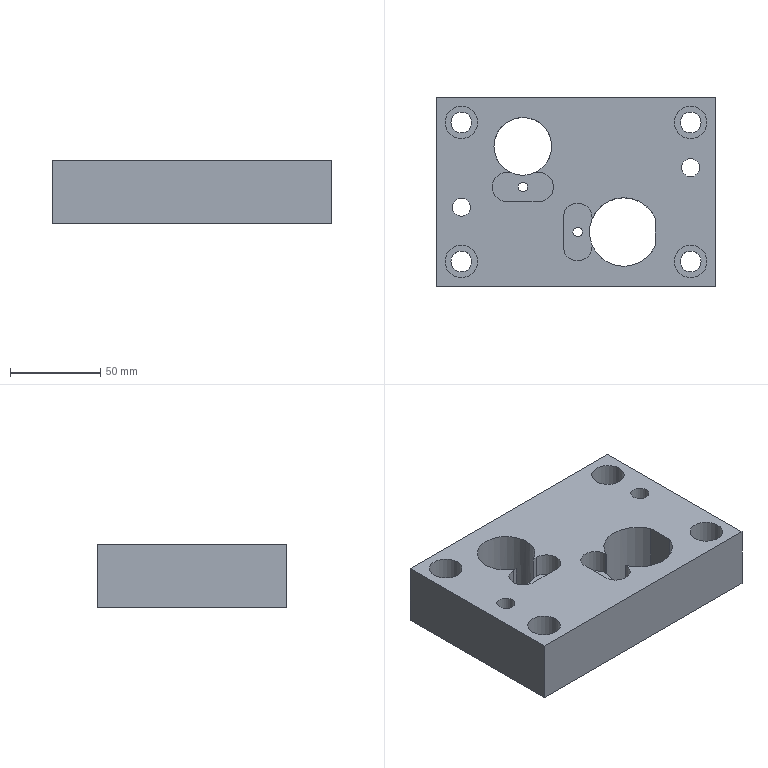Part | STEP file | lll_id4666_x_t | 1 solid | 38 faces | box 155 x 105 x 35 mm | volume 461543 mm3 | plane 19 | cylinder 19 | commonest cylinder face diameters 11.509 x4 16 x4 18.008 x4 5.206 x2 10 x2 38 x2
STEP:
#1=CARTESIAN_POINT('',(475.37,-354.819,-13.));
#2=VERTEX_POINT('',#1);
#3=CARTESIAN_POINT('',(474.87,-353.503,-13.));
#4=VERTEX_POINT('',#3);
#5=CARTESIAN_POINT('',(492.87,-347.42,-13.));
#6=DIRECTION('',(0.,0.,-1.));
#7=DIRECTION('',(1.,0.,0.));
#8=AXIS2_PLACEMENT_3D('',#5,#6,#7);
#9=CIRCLE('',#8,19.);
#10=EDGE_CURVE('',#2,#4,#9,.T.);
#11=ORIENTED_EDGE('',*,*,#10,.T.);
#12=CARTESIAN_POINT('',(475.37,-340.021,-13.));
#13=VERTEX_POINT('',#12);
#14=CARTESIAN_POINT('',(492.87,-347.42,-13.));
#15=DIRECTION('',(0.,0.,-1.));
#16=DIRECTION('',(1.,0.,0.));
#17=AXIS2_PLACEMENT_3D('',#14,#15,#16);
#18=CIRCLE('',#17,19.);
#19=EDGE_CURVE('',#4,#13,#18,.T.);
#20=ORIENTED_EDGE('',*,*,#19,.T.);
#21=CARTESIAN_POINT('',(475.37,-339.42,-13.));
#22=VERTEX_POINT('',#21);
#23=CARTESIAN_POINT('',(475.37,-339.42,-13.));
#24=DIRECTION('',(0.,1.,0.));
#25=VECTOR('',#24,1.);
#26=LINE('',#23,#25);
#27=EDGE_CURVE('',#13,#22,#26,.T.);
#28=ORIENTED_EDGE('',*,*,#27,.T.);
#29=CARTESIAN_POINT('',(459.37,-339.42,-13.));
#30=VERTEX_POINT('',#29);
#31=CARTESIAN_POINT('',(467.37,-339.42,-13.));
#32=DIRECTION('',(0.,0.,-1.));
#33=DIRECTION('',(1.,0.,0.));
#34=AXIS2_PLACEMENT_3D('',#31,#32,#33);
#35=CIRCLE('',#34,8.);
#36=EDGE_CURVE('',#30,#22,#35,.T.);
#37=ORIENTED_EDGE('',*,*,#36,.F.);
#38=CARTESIAN_POINT('',(459.37,-355.42,-13.));
#39=VERTEX_POINT('',#38);
#40=CARTESIAN_POINT('',(459.37,-339.42,-13.));
#41=DIRECTION('',(0.,1.,0.));
#42=VECTOR('',#41,1.);
#43=LINE('',#40,#42);
#44=EDGE_CURVE('',#39,#30,#43,.T.);
#45=ORIENTED_EDGE('',*,*,#44,.F.);
#46=CARTESIAN_POINT('',(475.37,-355.42,-13.));
#47=VERTEX_POINT('',#46);
#48=CARTESIAN_POINT('',(467.37,-355.42,-13.));
#49=DIRECTION('',(0.,0.,-1.));
#50=DIRECTION('',(1.,0.,0.));
#51=AXIS2_PLACEMENT_3D('',#48,#49,#50);
#52=CIRCLE('',#51,8.);
#53=EDGE_CURVE('',#47,#39,#52,.T.);
#54=ORIENTED_EDGE('',*,*,#53,.F.);
#55=CARTESIAN_POINT('',(475.37,-339.42,-13.));
#56=DIRECTION('',(0.,1.,0.));
#57=VECTOR('',#56,1.);
#58=LINE('',#55,#57);
#59=EDGE_CURVE('',#47,#2,#58,.T.);
#60=ORIENTED_EDGE('',*,*,#59,.T.);
#61=EDGE_LOOP('',(#11,#20,#28,#37,#45,#54,#60));
#62=FACE_BOUND('',#61,.T.);
#63=CARTESIAN_POINT('',(469.973,-347.42,-13.));
#64=VERTEX_POINT('',#63);
#65=CARTESIAN_POINT('',(467.37,-347.42,-13.));
#66=DIRECTION('',(0.,0.,-1.));
#67=DIRECTION('',(1.,0.,0.));
#68=AXIS2_PLACEMENT_3D('',#65,#66,#67);
#69=CIRCLE('',#68,2.603);
#70=EDGE_CURVE('',#64,#64,#69,.T.);
#71=ORIENTED_EDGE('',*,*,#70,.T.);
#72=EDGE_LOOP('',(#71));
#73=FACE_BOUND('',#72,.T.);
#74=CARTESIAN_POINT('',(467.37,-339.42,-13.));
#75=DIRECTION('',(0.,0.,1.));
#76=DIRECTION('',(1.,0.,0.));
#77=AXIS2_PLACEMENT_3D('',#74,#75,#76);
#78=PLANE('',#77);
#79=ADVANCED_FACE('',(#62,#73),#78,.T.);
#80=CARTESIAN_POINT('',(443.764,-314.5,-13.));
#81=VERTEX_POINT('',#80);
#82=CARTESIAN_POINT('',(430.236,-314.5,-13.));
#83=VERTEX_POINT('',#82);
#84=CARTESIAN_POINT('',(437.,-300.,-13.));
#85=DIRECTION('',(0.,0.,-1.));
#86=DIRECTION('',(1.,0.,0.));
#87=AXIS2_PLACEMENT_3D('',#84,#85,#86);
#88=CIRCLE('',#87,16.);
#89=EDGE_CURVE('',#81,#83,#88,.T.);
#90=ORIENTED_EDGE('',*,*,#89,.T.);
#91=CARTESIAN_POINT('',(428.,-314.5,-13.));
#92=VERTEX_POINT('',#91);
#93=CARTESIAN_POINT('',(428.,-314.5,-13.));
#94=DIRECTION('',(-1.,0.,0.));
#95=VECTOR('',#94,1.);
#96=LINE('',#93,#95);
#97=EDGE_CURVE('',#83,#92,#96,.T.);
#98=ORIENTED_EDGE('',*,*,#97,.T.);
#99=CARTESIAN_POINT('',(428.,-330.5,-13.));
#100=VERTEX_POINT('',#99);
#101=CARTESIAN_POINT('',(428.,-322.5,-13.));
#102=DIRECTION('',(0.,0.,-1.));
#103=DIRECTION('',(1.,0.,0.));
#104=AXIS2_PLACEMENT_3D('',#101,#102,#103);
#105=CIRCLE('',#104,8.);
#106=EDGE_CURVE('',#100,#92,#105,.T.);
#107=ORIENTED_EDGE('',*,*,#106,.F.);
#108=CARTESIAN_POINT('',(446.,-330.5,-13.));
#109=VERTEX_POINT('',#108);
#110=CARTESIAN_POINT('',(428.,-330.5,-13.));
#111=DIRECTION('',(-1.,0.,0.));
#112=VECTOR('',#111,1.);
#113=LINE('',#110,#112);
#114=EDGE_CURVE('',#109,#100,#113,.T.);
#115=ORIENTED_EDGE('',*,*,#114,.F.);
#116=CARTESIAN_POINT('',(446.,-314.5,-13.));
#117=VERTEX_POINT('',#116);
#118=CARTESIAN_POINT('',(446.,-322.5,-13.));
#119=DIRECTION('',(0.,0.,-1.));
#120=DIRECTION('',(1.,0.,0.));
#121=AXIS2_PLACEMENT_3D('',#118,#119,#120);
#122=CIRCLE('',#121,8.);
#123=EDGE_CURVE('',#117,#109,#122,.T.);
#124=ORIENTED_EDGE('',*,*,#123,.F.);
#125=CARTESIAN_POINT('',(428.,-314.5,-13.));
#126=DIRECTION('',(-1.,0.,0.));
#127=VECTOR('',#126,1.);
#128=LINE('',#125,#127);
#129=EDGE_CURVE('',#117,#81,#128,.T.);
#130=ORIENTED_EDGE('',*,*,#129,.T.);
#131=EDGE_LOOP('',(#90,#98,#107,#115,#124,#130));
#132=FACE_BOUND('',#131,.T.);
#133=CARTESIAN_POINT('',(439.603,-322.5,-13.));
#134=VERTEX_POINT('',#133);
#135=CARTESIAN_POINT('',(437.,-322.5,-13.));
#136=DIRECTION('',(0.,0.,-1.));
#137=DIRECTION('',(1.,0.,0.));
#138=AXIS2_PLACEMENT_3D('',#135,#136,#137);
#139=CIRCLE('',#138,2.603);
#140=EDGE_CURVE('',#134,#134,#139,.T.);
#141=ORIENTED_EDGE('',*,*,#140,.T.);
#142=EDGE_LOOP('',(#141));
#143=FACE_BOUND('',#142,.T.);
#144=CARTESIAN_POINT('',(428.,-322.5,-13.));
#145=DIRECTION('',(0.,0.,1.));
#146=DIRECTION('',(1.,0.,0.));
#147=AXIS2_PLACEMENT_3D('',#144,#145,#146);
#148=PLANE('',#147);
#149=ADVANCED_FACE('',(#132,#143),#148,.T.);
#150=CARTESIAN_POINT('',(475.37,-340.021,0.));
#151=VERTEX_POINT('',#150);
#152=CARTESIAN_POINT('',(475.37,-340.021,-15.));
#153=DIRECTION('',(0.,0.,1.));
#154=VECTOR('',#153,1.);
#155=LINE('',#152,#154);
#156=EDGE_CURVE('',#13,#151,#155,.T.);
#157=ORIENTED_EDGE('',*,*,#156,.F.);
#158=ORIENTED_EDGE('',*,*,#19,.F.);
#159=CARTESIAN_POINT('',(474.87,-353.503,-35.));
#160=VERTEX_POINT('',#159);
#161=CARTESIAN_POINT('',(474.87,-353.503,-15.));
#162=DIRECTION('',(0.,0.,1.));
#163=VECTOR('',#162,1.);
#164=LINE('',#161,#163);
#165=EDGE_CURVE('',#160,#4,#164,.T.);
#166=ORIENTED_EDGE('',*,*,#165,.F.);
#167=CARTESIAN_POINT('',(510.37,-340.021,-35.));
#168=VERTEX_POINT('',#167);
#169=CARTESIAN_POINT('',(492.87,-347.42,-35.));
#170=DIRECTION('',(0.,0.,1.));
#171=DIRECTION('',(-1.,0.,0.));
#172=AXIS2_PLACEMENT_3D('',#169,#170,#171);
#173=CIRCLE('',#172,19.);
#174=EDGE_CURVE('',#168,#160,#173,.T.);
#175=ORIENTED_EDGE('',*,*,#174,.F.);
#176=CARTESIAN_POINT('',(510.37,-340.021,0.));
#177=VERTEX_POINT('',#176);
#178=CARTESIAN_POINT('',(510.37,-340.021,0.));
#179=DIRECTION('',(0.,0.,-1.));
#180=VECTOR('',#179,1.);
#181=LINE('',#178,#180);
#182=EDGE_CURVE('',#177,#168,#181,.T.);
#183=ORIENTED_EDGE('',*,*,#182,.F.);
#184=CARTESIAN_POINT('',(492.87,-347.42,0.));
#185=DIRECTION('',(0.,0.,1.));
#186=DIRECTION('',(-1.,0.,0.));
#187=AXIS2_PLACEMENT_3D('',#184,#185,#186);
#188=CIRCLE('',#187,19.);
#189=EDGE_CURVE('',#177,#151,#188,.T.);
#190=ORIENTED_EDGE('',*,*,#189,.T.);
#191=EDGE_LOOP('',(#157,#158,#166,#175,#183,#190));
#192=FACE_OUTER_BOUND('',#191,.T.);
#193=CARTESIAN_POINT('',(492.87,-347.42,-15.));
#194=DIRECTION('',(0.,0.,-1.));
#195=DIRECTION('',(0.,1.,0.));
#196=AXIS2_PLACEMENT_3D('',#193,#194,#195);
#197=CYLINDRICAL_SURFACE('',#196,19.);
#198=ADVANCED_FACE('',(#192),#197,.F.);
#199=CARTESIAN_POINT('',(510.37,-354.819,0.));
#200=VERTEX_POINT('',#199);
#201=CARTESIAN_POINT('',(510.37,-354.819,0.));
#202=DIRECTION('',(0.,1.,0.));
#203=VECTOR('',#202,1.);
#204=LINE('',#201,#203);
#205=EDGE_CURVE('',#200,#177,#204,.T.);
#206=ORIENTED_EDGE('',*,*,#205,.F.);
#207=CARTESIAN_POINT('',(475.37,-354.819,0.));
#208=VERTEX_POINT('',#207);
#209=CARTESIAN_POINT('',(492.87,-347.42,0.));
#210=DIRECTION('',(0.,0.,1.));
#211=DIRECTION('',(-1.,0.,0.));
#212=AXIS2_PLACEMENT_3D('',#209,#210,#211);
#213=CIRCLE('',#212,19.);
#214=EDGE_CURVE('',#208,#200,#213,.T.);
#215=ORIENTED_EDGE('',*,*,#214,.F.);
#216=CARTESIAN_POINT('',(475.37,-355.42,0.));
#217=VERTEX_POINT('',#216);
#218=CARTESIAN_POINT('',(475.37,-325.25,0.));
#219=DIRECTION('',(0.,-1.,0.));
#220=VECTOR('',#219,1.);
#221=LINE('',#218,#220);
#222=EDGE_CURVE('',#208,#217,#221,.T.);
#223=ORIENTED_EDGE('',*,*,#222,.T.);
#224=CARTESIAN_POINT('',(459.37,-355.42,0.));
#225=VERTEX_POINT('',#224);
#226=CARTESIAN_POINT('',(467.37,-355.42,0.));
#227=DIRECTION('',(0.,0.,1.));
#228=DIRECTION('',(1.,0.,0.));
#229=AXIS2_PLACEMENT_3D('',#226,#227,#228);
#230=CIRCLE('',#229,8.);
#231=EDGE_CURVE('',#225,#217,#230,.T.);
#232=ORIENTED_EDGE('',*,*,#231,.F.);
#233=CARTESIAN_POINT('',(459.37,-339.42,0.));
#234=VERTEX_POINT('',#233);
#235=CARTESIAN_POINT('',(459.37,-325.25,0.));
#236=DIRECTION('',(0.,-1.,0.));
#237=VECTOR('',#236,1.);
#238=LINE('',#235,#237);
#239=EDGE_CURVE('',#234,#225,#238,.T.);
#240=ORIENTED_EDGE('',*,*,#239,.F.);
#241=CARTESIAN_POINT('',(475.37,-339.42,0.));
#242=VERTEX_POINT('',#241);
#243=CARTESIAN_POINT('',(467.37,-339.42,0.));
#244=DIRECTION('',(0.,0.,1.));
#245=DIRECTION('',(1.,0.,0.));
#246=AXIS2_PLACEMENT_3D('',#243,#244,#245);
#247=CIRCLE('',#246,8.);
#248=EDGE_CURVE('',#242,#234,#247,.T.);
#249=ORIENTED_EDGE('',*,*,#248,.F.);
#250=CARTESIAN_POINT('',(475.37,-325.25,0.));
#251=DIRECTION('',(0.,-1.,0.));
#252=VECTOR('',#251,1.);
#253=LINE('',#250,#252);
#254=EDGE_CURVE('',#242,#151,#253,.T.);
#255=ORIENTED_EDGE('',*,*,#254,.T.);
#256=ORIENTED_EDGE('',*,*,#189,.F.);
#257=EDGE_LOOP('',(#206,#215,#223,#232,#240,#249,#255,#256));
#258=FACE_BOUND('',#257,.T.);
#259=CARTESIAN_POINT('',(428.,-314.5,0.));
#260=VERTEX_POINT('',#259);
#261=CARTESIAN_POINT('',(428.,-330.5,0.));
#262=VERTEX_POINT('',#261);
#263=CARTESIAN_POINT('',(428.,-322.5,0.));
#264=DIRECTION('',(0.,0.,1.));
#265=DIRECTION('',(1.,0.,0.));
#266=AXIS2_PLACEMENT_3D('',#263,#264,#265);
#267=CIRCLE('',#266,8.);
#268=EDGE_CURVE('',#260,#262,#267,.T.);
#269=ORIENTED_EDGE('',*,*,#268,.F.);
#270=CARTESIAN_POINT('',(430.236,-314.5,0.));
#271=VERTEX_POINT('',#270);
#272=CARTESIAN_POINT('',(466.435,-314.5,0.));
#273=DIRECTION('',(1.,0.,0.));
#274=VECTOR('',#273,1.);
#275=LINE('',#272,#274);
#276=EDGE_CURVE('',#260,#271,#275,.T.);
#277=ORIENTED_EDGE('',*,*,#276,.T.);
#278=CARTESIAN_POINT('',(443.764,-314.5,0.));
#279=VERTEX_POINT('',#278);
#280=CARTESIAN_POINT('',(437.,-300.,0.));
#281=DIRECTION('',(0.,0.,1.));
#282=DIRECTION('',(-1.,0.,0.));
#283=AXIS2_PLACEMENT_3D('',#280,#281,#282);
#284=CIRCLE('',#283,16.);
#285=EDGE_CURVE('',#279,#271,#284,.T.);
#286=ORIENTED_EDGE('',*,*,#285,.F.);
#287=CARTESIAN_POINT('',(446.,-314.5,0.));
#288=VERTEX_POINT('',#287);
#289=CARTESIAN_POINT('',(466.435,-314.5,0.));
#290=DIRECTION('',(1.,0.,0.));
#291=VECTOR('',#290,1.);
#292=LINE('',#289,#291);
#293=EDGE_CURVE('',#279,#288,#292,.T.);
#294=ORIENTED_EDGE('',*,*,#293,.T.);
#295=CARTESIAN_POINT('',(446.,-330.5,0.));
#296=VERTEX_POINT('',#295);
#297=CARTESIAN_POINT('',(446.,-322.5,0.));
#298=DIRECTION('',(0.,0.,1.));
#299=DIRECTION('',(1.,0.,0.));
#300=AXIS2_PLACEMENT_3D('',#297,#298,#299);
#301=CIRCLE('',#300,8.);
#302=EDGE_CURVE('',#296,#288,#301,.T.);
#303=ORIENTED_EDGE('',*,*,#302,.F.);
#304=CARTESIAN_POINT('',(466.435,-330.5,0.));
#305=DIRECTION('',(1.,0.,0.));
#306=VECTOR('',#305,1.);
#307=LINE('',#304,#306);
#308=EDGE_CURVE('',#262,#296,#307,.T.);
#309=ORIENTED_EDGE('',*,*,#308,.F.);
#310=EDGE_LOOP('',(#269,#277,#286,#294,#303,#309));
#311=FACE_BOUND('',#310,.T.);
#312=CARTESIAN_POINT('',(393.931,-363.75,0.));
#313=VERTEX_POINT('',#312);
#314=CARTESIAN_POINT('',(402.935,-363.75,0.));
#315=DIRECTION('',(0.,0.,1.));
#316=DIRECTION('',(-1.,0.,0.));
#317=AXIS2_PLACEMENT_3D('',#314,#315,#316);
#318=CIRCLE('',#317,9.004);
#319=EDGE_CURVE('',#313,#313,#318,.T.);
#320=ORIENTED_EDGE('',*,*,#319,.F.);
#321=EDGE_LOOP('',(#320));
#322=FACE_BOUND('',#321,.T.);
#323=CARTESIAN_POINT('',(520.931,-286.75,0.));
#324=VERTEX_POINT('',#323);
#325=CARTESIAN_POINT('',(529.935,-286.75,0.));
#326=DIRECTION('',(0.,0.,1.));
#327=DIRECTION('',(-1.,0.,0.));
#328=AXIS2_PLACEMENT_3D('',#325,#326,#327);
#329=CIRCLE('',#328,9.004);
#330=EDGE_CURVE('',#324,#324,#329,.T.);
#331=ORIENTED_EDGE('',*,*,#330,.F.);
#332=EDGE_LOOP('',(#331));
#333=FACE_BOUND('',#332,.T.);
#334=CARTESIAN_POINT('',(388.935,-377.75,0.));
#335=VERTEX_POINT('',#334);
#336=CARTESIAN_POINT('',(543.935,-377.75,0.));
#337=VERTEX_POINT('',#336);
#338=CARTESIAN_POINT('',(466.435,-377.75,0.));
#339=DIRECTION('',(1.,0.,0.));
#340=VECTOR('',#339,1.);
#341=LINE('',#338,#340);
#342=EDGE_CURVE('',#335,#337,#341,.T.);
#343=ORIENTED_EDGE('',*,*,#342,.T.);
#344=CARTESIAN_POINT('',(543.935,-272.75,0.));
#345=VERTEX_POINT('',#344);
#346=CARTESIAN_POINT('',(543.935,-325.25,0.));
#347=DIRECTION('',(0.,1.,0.));
#348=VECTOR('',#347,1.);
#349=LINE('',#346,#348);
#350=EDGE_CURVE('',#337,#345,#349,.T.);
#351=ORIENTED_EDGE('',*,*,#350,.T.);
#352=CARTESIAN_POINT('',(388.935,-272.75,0.));
#353=VERTEX_POINT('',#352);
#354=CARTESIAN_POINT('',(466.435,-272.75,0.));
#355=DIRECTION('',(-1.,0.,0.));
#356=VECTOR('',#355,1.);
#357=LINE('',#354,#356);
#358=EDGE_CURVE('',#345,#353,#357,.T.);
#359=ORIENTED_EDGE('',*,*,#358,.T.);
#360=CARTESIAN_POINT('',(388.935,-325.25,0.));
#361=DIRECTION('',(0.,-1.,0.));
#362=VECTOR('',#361,1.);
#363=LINE('',#360,#362);
#364=EDGE_CURVE('',#353,#335,#363,.T.);
#365=ORIENTED_EDGE('',*,*,#364,.T.);
#366=EDGE_LOOP('',(#343,#351,#359,#365));
#367=FACE_BOUND('',#366,.T.);
#368=CARTESIAN_POINT('',(520.931,-363.75,0.));
#369=VERTEX_POINT('',#368);
#370=CARTESIAN_POINT('',(529.935,-363.75,0.));
#371=DIRECTION('',(0.,0.,1.));
#372=DIRECTION('',(-1.,0.,0.));
#373=AXIS2_PLACEMENT_3D('',#370,#371,#372);
#374=CIRCLE('',#373,9.004);
#375=EDGE_CURVE('',#369,#369,#374,.T.);
#376=ORIENTED_EDGE('',*,*,#375,.F.);
#377=EDGE_LOOP('',(#376));
#378=FACE_BOUND('',#377,.T.);
#379=CARTESIAN_POINT('',(524.935,-311.75,0.));
#380=VERTEX_POINT('',#379);
#381=CARTESIAN_POINT('',(529.935,-311.75,0.));
#382=DIRECTION('',(0.,0.,-1.));
#383=DIRECTION('',(-1.,0.,0.));
#384=AXIS2_PLACEMENT_3D('',#381,#382,#383);
#385=CIRCLE('',#384,5.);
#386=EDGE_CURVE('',#380,#380,#385,.T.);
#387=ORIENTED_EDGE('',*,*,#386,.T.);
#388=EDGE_LOOP('',(#387));
#389=FACE_BOUND('',#388,.T.);
#390=CARTESIAN_POINT('',(393.931,-286.75,0.));
#391=VERTEX_POINT('',#390);
#392=CARTESIAN_POINT('',(402.935,-286.75,0.));
#393=DIRECTION('',(0.,0.,1.));
#394=DIRECTION('',(-1.,0.,0.));
#395=AXIS2_PLACEMENT_3D('',#392,#393,#394);
#396=CIRCLE('',#395,9.004);
#397=EDGE_CURVE('',#391,#391,#396,.T.);
#398=ORIENTED_EDGE('',*,*,#397,.F.);
#399=EDGE_LOOP('',(#398));
#400=FACE_BOUND('',#399,.T.);
#401=CARTESIAN_POINT('',(397.935,-333.75,0.));
#402=VERTEX_POINT('',#401);
#403=CARTESIAN_POINT('',(402.935,-333.75,0.));
#404=DIRECTION('',(0.,0.,-1.));
#405=DIRECTION('',(-1.,0.,0.));
#406=AXIS2_PLACEMENT_3D('',#403,#404,#405);
#407=CIRCLE('',#406,5.);
#408=EDGE_CURVE('',#402,#402,#407,.T.);
#409=ORIENTED_EDGE('',*,*,#408,.T.);
#410=EDGE_LOOP('',(#409));
#411=FACE_BOUND('',#410,.T.);
#412=CARTESIAN_POINT('',(466.435,-325.25,0.));
#413=DIRECTION('',(0.,0.,1.));
#414=DIRECTION('',(-1.,0.,0.));
#415=AXIS2_PLACEMENT_3D('',#412,#413,#414);
#416=PLANE('',#415);
#417=ADVANCED_FACE('',(#258,#311,#322,#333,#367,#378,#389,#400,#411),#416,.T.);
#418=CARTESIAN_POINT('',(430.236,-314.5,-15.));
#419=DIRECTION('',(0.,0.,1.));
#420=VECTOR('',#419,1.);
#421=LINE('',#418,#420);
#422=EDGE_CURVE('',#83,#271,#421,.T.);
#423=ORIENTED_EDGE('',*,*,#422,.F.);
#424=ORIENTED_EDGE('',*,*,#89,.F.);
#425=CARTESIAN_POINT('',(443.764,-314.5,-15.));
#426=DIRECTION('',(0.,0.,-1.));
#427=VECTOR('',#426,1.);
#428=LINE('',#425,#427);
#429=EDGE_CURVE('',#279,#81,#428,.T.);
#430=ORIENTED_EDGE('',*,*,#429,.F.);
#431=ORIENTED_EDGE('',*,*,#285,.T.);
#432=EDGE_LOOP('',(#423,#424,#430,#431));
#433=FACE_BOUND('',#432,.T.);
#434=CARTESIAN_POINT('',(421.,-300.,-35.));
#435=VERTEX_POINT('',#434);
#436=CARTESIAN_POINT('',(437.,-300.,-35.));
#437=DIRECTION('',(0.,0.,-1.));
#438=DIRECTION('',(-1.,0.,0.));
#439=AXIS2_PLACEMENT_3D('',#436,#437,#438);
#440=CIRCLE('',#439,16.);
#441=EDGE_CURVE('',#435,#435,#440,.T.);
#442=ORIENTED_EDGE('',*,*,#441,.T.);
#443=EDGE_LOOP('',(#442));
#444=FACE_BOUND('',#443,.T.);
#445=CARTESIAN_POINT('',(437.,-300.,-15.));
#446=DIRECTION('',(0.,0.,-1.));
#447=DIRECTION('',(0.,1.,0.));
#448=AXIS2_PLACEMENT_3D('',#445,#446,#447);
#449=CYLINDRICAL_SURFACE('',#448,16.);
#450=ADVANCED_FACE('',(#433,#444),#449,.F.);
#451=ORIENTED_EDGE('',*,*,#214,.T.);
#452=CARTESIAN_POINT('',(510.37,-354.819,-35.));
#453=VERTEX_POINT('',#452);
#454=CARTESIAN_POINT('',(510.37,-354.819,-35.));
#455=DIRECTION('',(0.,0.,1.));
#456=VECTOR('',#455,1.);
#457=LINE('',#454,#456);
#458=EDGE_CURVE('',#453,#200,#457,.T.);
#459=ORIENTED_EDGE('',*,*,#458,.F.);
#460=CARTESIAN_POINT('',(492.87,-347.42,-35.));
#461=DIRECTION('',(0.,0.,1.));
#462=DIRECTION('',(-1.,0.,0.));
#463=AXIS2_PLACEMENT_3D('',#460,#461,#462);
#464=CIRCLE('',#463,19.);
#465=EDGE_CURVE('',#160,#453,#464,.T.);
#466=ORIENTED_EDGE('',*,*,#465,.F.);
#467=ORIENTED_EDGE('',*,*,#165,.T.);
#468=ORIENTED_EDGE('',*,*,#10,.F.);
#469=CARTESIAN_POINT('',(475.37,-354.819,-15.));
#470=DIRECTION('',(0.,0.,-1.));
#471=VECTOR('',#470,1.);
#472=LINE('',#469,#471);
#473=EDGE_CURVE('',#208,#2,#472,.T.);
#474=ORIENTED_EDGE('',*,*,#473,.F.);
#475=EDGE_LOOP('',(#451,#459,#466,#467,#468,#474));
#476=FACE_OUTER_BOUND('',#475,.T.);
#477=CARTESIAN_POINT('',(492.87,-347.42,-15.));
#478=DIRECTION('',(0.,0.,-1.));
#479=DIRECTION('',(0.,1.,0.));
#480=AXIS2_PLACEMENT_3D('',#477,#478,#479);
#481=CYLINDRICAL_SURFACE('',#480,19.);
#482=ADVANCED_FACE('',(#476),#481,.F.);
#483=ORIENTED_EDGE('',*,*,#465,.T.);
#484=CARTESIAN_POINT('',(510.37,-340.021,-35.));
#485=DIRECTION('',(0.,-1.,0.));
#486=VECTOR('',#485,1.);
#487=LINE('',#484,#486);
#488=EDGE_CURVE('',#168,#453,#487,.T.);
#489=ORIENTED_EDGE('',*,*,#488,.F.);
#490=ORIENTED_EDGE('',*,*,#174,.T.);
#491=EDGE_LOOP('',(#483,#489,#490));
#492=FACE_BOUND('',#491,.T.);
#493=ORIENTED_EDGE('',*,*,#441,.F.);
#494=EDGE_LOOP('',(#493));
#495=FACE_BOUND('',#494,.T.);
#496=CARTESIAN_POINT('',(464.767,-347.42,-35.));
#497=VERTEX_POINT('',#496);
#498=CARTESIAN_POINT('',(467.37,-347.42,-35.));
#499=DIRECTION('',(0.,0.,-1.));
#500=DIRECTION('',(-1.,0.,0.));
#501=AXIS2_PLACEMENT_3D('',#498,#499,#500);
#502=CIRCLE('',#501,2.603);
#503=EDGE_CURVE('',#497,#497,#502,.T.);
#504=ORIENTED_EDGE('',*,*,#503,.F.);
#505=EDGE_LOOP('',(#504));
#506=FACE_BOUND('',#505,.T.);
#507=CARTESIAN_POINT('',(434.397,-322.5,-35.));
#508=VERTEX_POINT('',#507);
#509=CARTESIAN_POINT('',(437.,-322.5,-35.));
#510=DIRECTION('',(0.,0.,-1.));
#511=DIRECTION('',(-1.,0.,0.));
#512=AXIS2_PLACEMENT_3D('',#509,#510,#511);
#513=CIRCLE('',#512,2.603);
#514=EDGE_CURVE('',#508,#508,#513,.T.);
#515=ORIENTED_EDGE('',*,*,#514,.F.);
#516=EDGE_LOOP('',(#515));
#517=FACE_BOUND('',#516,.T.);
#518=CARTESIAN_POINT('',(407.935,-333.75,-35.));
#519=VERTEX_POINT('',#518);
#520=CARTESIAN_POINT('',(402.935,-333.75,-35.));
#521=DIRECTION('',(0.,0.,1.));
#522=DIRECTION('',(1.,0.,0.));
#523=AXIS2_PLACEMENT_3D('',#520,#521,#522);
#524=CIRCLE('',#523,5.);
#525=EDGE_CURVE('',#519,#519,#524,.T.);
#526=ORIENTED_EDGE('',*,*,#525,.T.);
#527=EDGE_LOOP('',(#526));
#528=FACE_BOUND('',#527,.T.);
#529=CARTESIAN_POINT('',(408.69,-363.75,-35.));
#530=VERTEX_POINT('',#529);
#531=CARTESIAN_POINT('',(402.935,-363.75,-35.));
#532=DIRECTION('',(0.,0.,1.));
#533=DIRECTION('',(1.,0.,0.));
#534=AXIS2_PLACEMENT_3D('',#531,#532,#533);
#535=CIRCLE('',#534,5.755);
#536=EDGE_CURVE('',#530,#530,#535,.T.);
#537=ORIENTED_EDGE('',*,*,#536,.T.);
#538=EDGE_LOOP('',(#537));
#539=FACE_BOUND('',#538,.T.);
#540=CARTESIAN_POINT('',(408.69,-286.75,-35.));
#541=VERTEX_POINT('',#540);
#542=CARTESIAN_POINT('',(402.935,-286.75,-35.));
#543=DIRECTION('',(0.,0.,1.));
#544=DIRECTION('',(1.,0.,0.));
#545=AXIS2_PLACEMENT_3D('',#542,#543,#544);
#546=CIRCLE('',#545,5.755);
#547=EDGE_CURVE('',#541,#541,#546,.T.);
#548=ORIENTED_EDGE('',*,*,#547,.T.);
#549=EDGE_LOOP('',(#548));
#550=FACE_BOUND('',#549,.T.);
#551=CARTESIAN_POINT('',(534.935,-311.75,-35.));
#552=VERTEX_POINT('',#551);
#553=CARTESIAN_POINT('',(529.935,-311.75,-35.));
#554=DIRECTION('',(0.,0.,1.));
#555=DIRECTION('',(1.,0.,0.));
#556=AXIS2_PLACEMENT_3D('',#553,#554,#555);
#557=CIRCLE('',#556,5.);
#558=EDGE_CURVE('',#552,#552,#557,.T.);
#559=ORIENTED_EDGE('',*,*,#558,.T.);
#560=EDGE_LOOP('',(#559));
#561=FACE_BOUND('',#560,.T.);
#562=CARTESIAN_POINT('',(535.69,-286.75,-35.));
#563=VERTEX_POINT('',#562);
#564=CARTESIAN_POINT('',(529.935,-286.75,-35.));
#565=DIRECTION('',(0.,0.,1.));
#566=DIRECTION('',(1.,0.,0.));
#567=AXIS2_PLACEMENT_3D('',#564,#565,#566);
#568=CIRCLE('',#567,5.755);
#569=EDGE_CURVE('',#563,#563,#568,.T.);
#570=ORIENTED_EDGE('',*,*,#569,.T.);
#571=EDGE_LOOP('',(#570));
#572=FACE_BOUND('',#571,.T.);
#573=CARTESIAN_POINT('',(535.69,-363.75,-35.));
#574=VERTEX_POINT('',#573);
#575=CARTESIAN_POINT('',(529.935,-363.75,-35.));
#576=DIRECTION('',(0.,0.,1.));
#577=DIRECTION('',(1.,0.,0.));
#578=AXIS2_PLACEMENT_3D('',#575,#576,#577);
#579=CIRCLE('',#578,5.755);
#580=EDGE_CURVE('',#574,#574,#579,.T.);
#581=ORIENTED_EDGE('',*,*,#580,.T.);
#582=EDGE_LOOP('',(#581));
#583=FACE_BOUND('',#582,.T.);
#584=CARTESIAN_POINT('',(388.935,-377.75,-35.));
#585=VERTEX_POINT('',#584);
#586=CARTESIAN_POINT('',(388.935,-272.75,-35.));
#587=VERTEX_POINT('',#586);
#588=CARTESIAN_POINT('',(388.935,-325.25,-35.));
#589=DIRECTION('',(0.,1.,0.));
#590=VECTOR('',#589,1.);
#591=LINE('',#588,#590);
#592=EDGE_CURVE('',#585,#587,#591,.T.);
#593=ORIENTED_EDGE('',*,*,#592,.T.);
#594=CARTESIAN_POINT('',(543.935,-272.75,-35.));
#595=VERTEX_POINT('',#594);
#596=CARTESIAN_POINT('',(466.435,-272.75,-35.));
#597=DIRECTION('',(1.,0.,0.));
#598=VECTOR('',#597,1.);
#599=LINE('',#596,#598);
#600=EDGE_CURVE('',#587,#595,#599,.T.);
#601=ORIENTED_EDGE('',*,*,#600,.T.);
#602=CARTESIAN_POINT('',(543.935,-377.75,-35.));
#603=VERTEX_POINT('',#602);
#604=CARTESIAN_POINT('',(543.935,-325.25,-35.));
#605=DIRECTION('',(0.,-1.,0.));
#606=VECTOR('',#605,1.);
#607=LINE('',#604,#606);
#608=EDGE_CURVE('',#595,#603,#607,.T.);
#609=ORIENTED_EDGE('',*,*,#608,.T.);
#610=CARTESIAN_POINT('',(466.435,-377.75,-35.));
#611=DIRECTION('',(-1.,0.,0.));
#612=VECTOR('',#611,1.);
#613=LINE('',#610,#612);
#614=EDGE_CURVE('',#603,#585,#613,.T.);
#615=ORIENTED_EDGE('',*,*,#614,.T.);
#616=EDGE_LOOP('',(#593,#601,#609,#615));
#617=FACE_BOUND('',#616,.T.);
#618=CARTESIAN_POINT('',(466.435,-325.25,-35.));
#619=DIRECTION('',(0.,0.,-1.));
#620=DIRECTION('',(1.,0.,0.));
#621=AXIS2_PLACEMENT_3D('',#618,#619,#620);
#622=PLANE('',#621);
#623=ADVANCED_FACE('',(#492,#495,#506,#517,#528,#539,#550,#561,#572,#583,#617),#622,.T.);
#624=CARTESIAN_POINT('',(388.935,-377.75,-32.));
#625=DIRECTION('',(0.,0.,1.));
#626=VECTOR('',#625,1.);
#627=LINE('',#624,#626);
#628=EDGE_CURVE('',#585,#335,#627,.T.);
#629=ORIENTED_EDGE('',*,*,#628,.F.);
#630=ORIENTED_EDGE('',*,*,#614,.F.);
#631=CARTESIAN_POINT('',(543.935,-377.75,-32.));
#632=DIRECTION('',(0.,0.,1.));
#633=VECTOR('',#632,1.);
#634=LINE('',#631,#633);
#635=EDGE_CURVE('',#603,#337,#634,.T.);
#636=ORIENTED_EDGE('',*,*,#635,.T.);
#637=ORIENTED_EDGE('',*,*,#342,.F.);
#638=EDGE_LOOP('',(#629,#630,#636,#637));
#639=FACE_OUTER_BOUND('',#638,.T.);
#640=CARTESIAN_POINT('',(466.435,-377.75,-32.));
#641=DIRECTION('',(0.,-1.,0.));
#642=DIRECTION('',(0.,0.,-1.));
#643=AXIS2_PLACEMENT_3D('',#640,#641,#642);
#644=PLANE('',#643);
#645=ADVANCED_FACE('',(#639),#644,.T.);
#646=ORIENTED_EDGE('',*,*,#635,.F.);
#647=ORIENTED_EDGE('',*,*,#608,.F.);
#648=CARTESIAN_POINT('',(543.935,-272.75,-32.));
#649=DIRECTION('',(0.,0.,1.));
#650=VECTOR('',#649,1.);
#651=LINE('',#648,#650);
#652=EDGE_CURVE('',#595,#345,#651,.T.);
#653=ORIENTED_EDGE('',*,*,#652,.T.);
#654=ORIENTED_EDGE('',*,*,#350,.F.);
#655=EDGE_LOOP('',(#646,#647,#653,#654));
#656=FACE_OUTER_BOUND('',#655,.T.);
#657=CARTESIAN_POINT('',(543.935,-325.25,-32.));
#658=DIRECTION('',(1.,0.,0.));
#659=DIRECTION('',(0.,0.,1.));
#660=AXIS2_PLACEMENT_3D('',#657,#658,#659);
#661=PLANE('',#660);
#662=ADVANCED_FACE('',(#656),#661,.T.);
#663=ORIENTED_EDGE('',*,*,#652,.F.);
#664=ORIENTED_EDGE('',*,*,#600,.F.);
#665=CARTESIAN_POINT('',(388.935,-272.75,-32.));
#666=DIRECTION('',(0.,0.,1.));
#667=VECTOR('',#666,1.);
#668=LINE('',#665,#667);
#669=EDGE_CURVE('',#587,#353,#668,.T.);
#670=ORIENTED_EDGE('',*,*,#669,.T.);
#671=ORIENTED_EDGE('',*,*,#358,.F.);
#672=EDGE_LOOP('',(#663,#664,#670,#671));
#673=FACE_OUTER_BOUND('',#672,.T.);
#674=CARTESIAN_POINT('',(466.435,-272.75,-32.));
#675=DIRECTION('',(0.,1.,0.));
#676=DIRECTION('',(0.,0.,1.));
#677=AXIS2_PLACEMENT_3D('',#674,#675,#676);
#678=PLANE('',#677);
#679=ADVANCED_FACE('',(#673),#678,.T.);
#680=ORIENTED_EDGE('',*,*,#592,.F.);
#681=ORIENTED_EDGE('',*,*,#628,.T.);
#682=ORIENTED_EDGE('',*,*,#364,.F.);
#683=ORIENTED_EDGE('',*,*,#669,.F.);
#684=EDGE_LOOP('',(#680,#681,#682,#683));
#685=FACE_OUTER_BOUND('',#684,.T.);
#686=CARTESIAN_POINT('',(388.935,-325.25,-32.));
#687=DIRECTION('',(-1.,0.,0.));
#688=DIRECTION('',(0.,0.,-1.));
#689=AXIS2_PLACEMENT_3D('',#686,#687,#688);
#690=PLANE('',#689);
#691=ADVANCED_FACE('',(#685),#690,.T.);
#692=ORIENTED_EDGE('',*,*,#580,.F.);
#693=EDGE_LOOP('',(#692));
#694=FACE_BOUND('',#693,.T.);
#695=CARTESIAN_POINT('',(535.69,-363.75,-13.));
#696=VERTEX_POINT('',#695);
#697=CARTESIAN_POINT('',(529.935,-363.75,-13.));
#698=DIRECTION('',(0.,0.,1.));
#699=DIRECTION('',(1.,0.,0.));
#700=AXIS2_PLACEMENT_3D('',#697,#698,#699);
#701=CIRCLE('',#700,5.755);
#702=EDGE_CURVE('',#696,#696,#701,.T.);
#703=ORIENTED_EDGE('',*,*,#702,.T.);
#704=EDGE_LOOP('',(#703));
#705=FACE_BOUND('',#704,.T.);
#706=CARTESIAN_POINT('',(529.935,-363.75,2.));
#707=DIRECTION('',(0.,0.,-1.));
#708=DIRECTION('',(-1.,0.,0.));
#709=AXIS2_PLACEMENT_3D('',#706,#707,#708);
#710=CYLINDRICAL_SURFACE('',#709,5.755);
#711=ADVANCED_FACE('',(#694,#705),#710,.F.);
#712=ORIENTED_EDGE('',*,*,#702,.F.);
#713=EDGE_LOOP('',(#712));
#714=FACE_BOUND('',#713,.T.);
#715=CARTESIAN_POINT('',(520.931,-363.75,-13.));
#716=VERTEX_POINT('',#715);
#717=CARTESIAN_POINT('',(529.935,-363.75,-13.));
#718=DIRECTION('',(0.,0.,1.));
#719=DIRECTION('',(-1.,0.,0.));
#720=AXIS2_PLACEMENT_3D('',#717,#718,#719);
#721=CIRCLE('',#720,9.004);
#722=EDGE_CURVE('',#716,#716,#721,.T.);
#723=ORIENTED_EDGE('',*,*,#722,.T.);
#724=EDGE_LOOP('',(#723));
#725=FACE_BOUND('',#724,.T.);
#726=CARTESIAN_POINT('',(529.935,-363.75,-13.));
#727=DIRECTION('',(0.,0.,-1.));
#728=DIRECTION('',(1.,0.,0.));
#729=AXIS2_PLACEMENT_3D('',#726,#727,#728);
#730=PLANE('',#729);
#731=ADVANCED_FACE('',(#714,#725),#730,.F.);
#732=ORIENTED_EDGE('',*,*,#722,.F.);
#733=EDGE_LOOP('',(#732));
#734=FACE_BOUND('',#733,.T.);
#735=ORIENTED_EDGE('',*,*,#375,.T.);
#736=EDGE_LOOP('',(#735));
#737=FACE_BOUND('',#736,.T.);
#738=CARTESIAN_POINT('',(529.935,-363.75,0.));
#739=DIRECTION('',(0.,0.,-1.));
#740=DIRECTION('',(-1.,0.,0.));
#741=AXIS2_PLACEMENT_3D('',#738,#739,#740);
#742=CYLINDRICAL_SURFACE('',#741,9.004);
#743=ADVANCED_FACE('',(#734,#737),#742,.F.);
#744=ORIENTED_EDGE('',*,*,#569,.F.);
#745=EDGE_LOOP('',(#744));
#746=FACE_BOUND('',#745,.T.);
#747=CARTESIAN_POINT('',(535.69,-286.75,-13.));
#748=VERTEX_POINT('',#747);
#749=CARTESIAN_POINT('',(529.935,-286.75,-13.));
#750=DIRECTION('',(0.,0.,1.));
#751=DIRECTION('',(1.,0.,0.));
#752=AXIS2_PLACEMENT_3D('',#749,#750,#751);
#753=CIRCLE('',#752,5.755);
#754=EDGE_CURVE('',#748,#748,#753,.T.);
#755=ORIENTED_EDGE('',*,*,#754,.T.);
#756=EDGE_LOOP('',(#755));
#757=FACE_BOUND('',#756,.T.);
#758=CARTESIAN_POINT('',(529.935,-286.75,2.));
#759=DIRECTION('',(0.,0.,-1.));
#760=DIRECTION('',(-1.,0.,0.));
#761=AXIS2_PLACEMENT_3D('',#758,#759,#760);
#762=CYLINDRICAL_SURFACE('',#761,5.755);
#763=ADVANCED_FACE('',(#746,#757),#762,.F.);
#764=ORIENTED_EDGE('',*,*,#754,.F.);
#765=EDGE_LOOP('',(#764));
#766=FACE_BOUND('',#765,.T.);
#767=CARTESIAN_POINT('',(520.931,-286.75,-13.));
#768=VERTEX_POINT('',#767);
#769=CARTESIAN_POINT('',(529.935,-286.75,-13.));
#770=DIRECTION('',(0.,0.,1.));
#771=DIRECTION('',(-1.,0.,0.));
#772=AXIS2_PLACEMENT_3D('',#769,#770,#771);
#773=CIRCLE('',#772,9.004);
#774=EDGE_CURVE('',#768,#768,#773,.T.);
#775=ORIENTED_EDGE('',*,*,#774,.T.);
#776=EDGE_LOOP('',(#775));
#777=FACE_BOUND('',#776,.T.);
#778=CARTESIAN_POINT('',(529.935,-286.75,-13.));
#779=DIRECTION('',(0.,0.,-1.));
#780=DIRECTION('',(1.,0.,0.));
#781=AXIS2_PLACEMENT_3D('',#778,#779,#780);
#782=PLANE('',#781);
#783=ADVANCED_FACE('',(#766,#777),#782,.F.);
#784=ORIENTED_EDGE('',*,*,#774,.F.);
#785=EDGE_LOOP('',(#784));
#786=FACE_BOUND('',#785,.T.);
#787=ORIENTED_EDGE('',*,*,#330,.T.);
#788=EDGE_LOOP('',(#787));
#789=FACE_BOUND('',#788,.T.);
#790=CARTESIAN_POINT('',(529.935,-286.75,0.));
#791=DIRECTION('',(0.,0.,-1.));
#792=DIRECTION('',(-1.,0.,0.));
#793=AXIS2_PLACEMENT_3D('',#790,#791,#792);
#794=CYLINDRICAL_SURFACE('',#793,9.004);
#795=ADVANCED_FACE('',(#786,#789),#794,.F.);
#796=ORIENTED_EDGE('',*,*,#386,.F.);
#797=EDGE_LOOP('',(#796));
#798=FACE_BOUND('',#797,.T.);
#799=ORIENTED_EDGE('',*,*,#558,.F.);
#800=EDGE_LOOP('',(#799));
#801=FACE_BOUND('',#800,.T.);
#802=CARTESIAN_POINT('',(529.935,-311.75,2.));
#803=DIRECTION('',(0.,0.,-1.));
#804=DIRECTION('',(-1.,0.,0.));
#805=AXIS2_PLACEMENT_3D('',#802,#803,#804);
#806=CYLINDRICAL_SURFACE('',#805,5.);
#807=ADVANCED_FACE('',(#798,#801),#806,.F.);
#808=ORIENTED_EDGE('',*,*,#547,.F.);
#809=EDGE_LOOP('',(#808));
#810=FACE_BOUND('',#809,.T.);
#811=CARTESIAN_POINT('',(408.69,-286.75,-13.));
#812=VERTEX_POINT('',#811);
#813=CARTESIAN_POINT('',(402.935,-286.75,-13.));
#814=DIRECTION('',(0.,0.,1.));
#815=DIRECTION('',(1.,0.,0.));
#816=AXIS2_PLACEMENT_3D('',#813,#814,#815);
#817=CIRCLE('',#816,5.755);
#818=EDGE_CURVE('',#812,#812,#817,.T.);
#819=ORIENTED_EDGE('',*,*,#818,.T.);
#820=EDGE_LOOP('',(#819));
#821=FACE_BOUND('',#820,.T.);
#822=CARTESIAN_POINT('',(402.935,-286.75,2.));
#823=DIRECTION('',(0.,0.,-1.));
#824=DIRECTION('',(-1.,0.,0.));
#825=AXIS2_PLACEMENT_3D('',#822,#823,#824);
#826=CYLINDRICAL_SURFACE('',#825,5.755);
#827=ADVANCED_FACE('',(#810,#821),#826,.F.);
#828=ORIENTED_EDGE('',*,*,#818,.F.);
#829=EDGE_LOOP('',(#828));
#830=FACE_BOUND('',#829,.T.);
#831=CARTESIAN_POINT('',(393.931,-286.75,-13.));
#832=VERTEX_POINT('',#831);
#833=CARTESIAN_POINT('',(402.935,-286.75,-13.));
#834=DIRECTION('',(0.,0.,1.));
#835=DIRECTION('',(-1.,0.,0.));
#836=AXIS2_PLACEMENT_3D('',#833,#834,#835);
#837=CIRCLE('',#836,9.004);
#838=EDGE_CURVE('',#832,#832,#837,.T.);
#839=ORIENTED_EDGE('',*,*,#838,.T.);
#840=EDGE_LOOP('',(#839));
#841=FACE_BOUND('',#840,.T.);
#842=CARTESIAN_POINT('',(402.935,-286.75,-13.));
#843=DIRECTION('',(0.,0.,-1.));
#844=DIRECTION('',(1.,0.,0.));
#845=AXIS2_PLACEMENT_3D('',#842,#843,#844);
#846=PLANE('',#845);
#847=ADVANCED_FACE('',(#830,#841),#846,.F.);
#848=ORIENTED_EDGE('',*,*,#838,.F.);
#849=EDGE_LOOP('',(#848));
#850=FACE_BOUND('',#849,.T.);
#851=ORIENTED_EDGE('',*,*,#397,.T.);
#852=EDGE_LOOP('',(#851));
#853=FACE_BOUND('',#852,.T.);
#854=CARTESIAN_POINT('',(402.935,-286.75,0.));
#855=DIRECTION('',(0.,0.,-1.));
#856=DIRECTION('',(-1.,0.,0.));
#857=AXIS2_PLACEMENT_3D('',#854,#855,#856);
#858=CYLINDRICAL_SURFACE('',#857,9.004);
#859=ADVANCED_FACE('',(#850,#853),#858,.F.);
#860=ORIENTED_EDGE('',*,*,#536,.F.);
#861=EDGE_LOOP('',(#860));
#862=FACE_BOUND('',#861,.T.);
#863=CARTESIAN_POINT('',(408.69,-363.75,-13.));
#864=VERTEX_POINT('',#863);
#865=CARTESIAN_POINT('',(402.935,-363.75,-13.));
#866=DIRECTION('',(0.,0.,1.));
#867=DIRECTION('',(1.,0.,0.));
#868=AXIS2_PLACEMENT_3D('',#865,#866,#867);
#869=CIRCLE('',#868,5.755);
#870=EDGE_CURVE('',#864,#864,#869,.T.);
#871=ORIENTED_EDGE('',*,*,#870,.T.);
#872=EDGE_LOOP('',(#871));
#873=FACE_BOUND('',#872,.T.);
#874=CARTESIAN_POINT('',(402.935,-363.75,2.));
#875=DIRECTION('',(0.,0.,-1.));
#876=DIRECTION('',(-1.,0.,0.));
#877=AXIS2_PLACEMENT_3D('',#874,#875,#876);
#878=CYLINDRICAL_SURFACE('',#877,5.755);
#879=ADVANCED_FACE('',(#862,#873),#878,.F.);
#880=ORIENTED_EDGE('',*,*,#870,.F.);
#881=EDGE_LOOP('',(#880));
#882=FACE_BOUND('',#881,.T.);
#883=CARTESIAN_POINT('',(393.931,-363.75,-13.));
#884=VERTEX_POINT('',#883);
#885=CARTESIAN_POINT('',(402.935,-363.75,-13.));
#886=DIRECTION('',(0.,0.,1.));
#887=DIRECTION('',(-1.,0.,0.));
#888=AXIS2_PLACEMENT_3D('',#885,#886,#887);
#889=CIRCLE('',#888,9.004);
#890=EDGE_CURVE('',#884,#884,#889,.T.);
#891=ORIENTED_EDGE('',*,*,#890,.T.);
#892=EDGE_LOOP('',(#891));
#893=FACE_BOUND('',#892,.T.);
#894=CARTESIAN_POINT('',(402.935,-363.75,-13.));
#895=DIRECTION('',(0.,0.,-1.));
#896=DIRECTION('',(1.,0.,0.));
#897=AXIS2_PLACEMENT_3D('',#894,#895,#896);
#898=PLANE('',#897);
#899=ADVANCED_FACE('',(#882,#893),#898,.F.);
#900=ORIENTED_EDGE('',*,*,#890,.F.);
#901=EDGE_LOOP('',(#900));
#902=FACE_BOUND('',#901,.T.);
#903=ORIENTED_EDGE('',*,*,#319,.T.);
#904=EDGE_LOOP('',(#903));
#905=FACE_BOUND('',#904,.T.);
#906=CARTESIAN_POINT('',(402.935,-363.75,0.));
#907=DIRECTION('',(0.,0.,-1.));
#908=DIRECTION('',(-1.,0.,0.));
#909=AXIS2_PLACEMENT_3D('',#906,#907,#908);
#910=CYLINDRICAL_SURFACE('',#909,9.004);
#911=ADVANCED_FACE('',(#902,#905),#910,.F.);
#912=ORIENTED_EDGE('',*,*,#408,.F.);
#913=EDGE_LOOP('',(#912));
#914=FACE_BOUND('',#913,.T.);
#915=ORIENTED_EDGE('',*,*,#525,.F.);
#916=EDGE_LOOP('',(#915));
#917=FACE_BOUND('',#916,.T.);
#918=CARTESIAN_POINT('',(402.935,-333.75,2.));
#919=DIRECTION('',(0.,0.,-1.));
#920=DIRECTION('',(-1.,0.,0.));
#921=AXIS2_PLACEMENT_3D('',#918,#919,#920);
#922=CYLINDRICAL_SURFACE('',#921,5.);
#923=ADVANCED_FACE('',(#914,#917),#922,.F.);
#924=CARTESIAN_POINT('',(475.37,-339.42,-1.));
#925=DIRECTION('',(0.,0.,-1.));
#926=VECTOR('',#925,1.);
#927=LINE('',#924,#926);
#928=EDGE_CURVE('',#242,#22,#927,.T.);
#929=ORIENTED_EDGE('',*,*,#928,.T.);
#930=ORIENTED_EDGE('',*,*,#27,.F.);
#931=ORIENTED_EDGE('',*,*,#156,.T.);
#932=ORIENTED_EDGE('',*,*,#254,.F.);
#933=EDGE_LOOP('',(#929,#930,#931,#932));
#934=FACE_OUTER_BOUND('',#933,.T.);
#935=CARTESIAN_POINT('',(475.37,0.,0.));
#936=DIRECTION('',(-1.,0.,0.));
#937=DIRECTION('',(0.,0.,1.));
#938=AXIS2_PLACEMENT_3D('',#935,#936,#937);
#939=PLANE('',#938);
#940=ADVANCED_FACE('',(#934),#939,.T.);
#941=ORIENTED_EDGE('',*,*,#473,.T.);
#942=ORIENTED_EDGE('',*,*,#59,.F.);
#943=CARTESIAN_POINT('',(475.37,-355.42,-7.));
#944=DIRECTION('',(0.,0.,1.));
#945=VECTOR('',#944,1.);
#946=LINE('',#943,#945);
#947=EDGE_CURVE('',#47,#217,#946,.T.);
#948=ORIENTED_EDGE('',*,*,#947,.T.);
#949=ORIENTED_EDGE('',*,*,#222,.F.);
#950=EDGE_LOOP('',(#941,#942,#948,#949));
#951=FACE_OUTER_BOUND('',#950,.T.);
#952=CARTESIAN_POINT('',(475.37,0.,0.));
#953=DIRECTION('',(-1.,0.,0.));
#954=DIRECTION('',(0.,0.,1.));
#955=AXIS2_PLACEMENT_3D('',#952,#953,#954);
#956=PLANE('',#955);
#957=ADVANCED_FACE('',(#951),#956,.T.);
#958=ORIENTED_EDGE('',*,*,#239,.T.);
#959=CARTESIAN_POINT('',(459.37,-355.42,-1.));
#960=DIRECTION('',(0.,0.,1.));
#961=VECTOR('',#960,1.);
#962=LINE('',#959,#961);
#963=EDGE_CURVE('',#39,#225,#962,.T.);
#964=ORIENTED_EDGE('',*,*,#963,.F.);
#965=ORIENTED_EDGE('',*,*,#44,.T.);
#966=CARTESIAN_POINT('',(459.37,-339.42,-1.));
#967=DIRECTION('',(0.,0.,-1.));
#968=VECTOR('',#967,1.);
#969=LINE('',#966,#968);
#970=EDGE_CURVE('',#234,#30,#969,.T.);
#971=ORIENTED_EDGE('',*,*,#970,.F.);
#972=EDGE_LOOP('',(#958,#964,#965,#971));
#973=FACE_OUTER_BOUND('',#972,.T.);
#974=CARTESIAN_POINT('',(459.37,0.,0.));
#975=DIRECTION('',(-1.,0.,0.));
#976=DIRECTION('',(0.,0.,1.));
#977=AXIS2_PLACEMENT_3D('',#974,#975,#976);
#978=PLANE('',#977);
#979=ADVANCED_FACE('',(#973),#978,.F.);
#980=ORIENTED_EDGE('',*,*,#248,.T.);
#981=ORIENTED_EDGE('',*,*,#970,.T.);
#982=ORIENTED_EDGE('',*,*,#36,.T.);
#983=ORIENTED_EDGE('',*,*,#928,.F.);
#984=EDGE_LOOP('',(#980,#981,#982,#983));
#985=FACE_OUTER_BOUND('',#984,.T.);
#986=CARTESIAN_POINT('',(467.37,-339.42,-1.));
#987=DIRECTION('',(0.,0.,-1.));
#988=DIRECTION('',(1.,0.,0.));
#989=AXIS2_PLACEMENT_3D('',#986,#987,#988);
#990=CYLINDRICAL_SURFACE('',#989,8.);
#991=ADVANCED_FACE('',(#985),#990,.F.);
#992=ORIENTED_EDGE('',*,*,#231,.T.);
#993=ORIENTED_EDGE('',*,*,#947,.F.);
#994=ORIENTED_EDGE('',*,*,#53,.T.);
#995=ORIENTED_EDGE('',*,*,#963,.T.);
#996=EDGE_LOOP('',(#992,#993,#994,#995));
#997=FACE_OUTER_BOUND('',#996,.T.);
#998=CARTESIAN_POINT('',(467.37,-355.42,-1.));
#999=DIRECTION('',(0.,0.,-1.));
#1000=DIRECTION('',(1.,0.,0.));
#1001=AXIS2_PLACEMENT_3D('',#998,#999,#1000);
#1002=CYLINDRICAL_SURFACE('',#1001,8.);
#1003=ADVANCED_FACE('',(#997),#1002,.F.);
#1004=CARTESIAN_POINT('',(428.,-314.5,-1.));
#1005=DIRECTION('',(0.,0.,-1.));
#1006=VECTOR('',#1005,1.);
#1007=LINE('',#1004,#1006);
#1008=EDGE_CURVE('',#260,#92,#1007,.T.);
#1009=ORIENTED_EDGE('',*,*,#1008,.T.);
#1010=ORIENTED_EDGE('',*,*,#97,.F.);
#1011=ORIENTED_EDGE('',*,*,#422,.T.);
#1012=ORIENTED_EDGE('',*,*,#276,.F.);
#1013=EDGE_LOOP('',(#1009,#1010,#1011,#1012));
#1014=FACE_OUTER_BOUND('',#1013,.T.);
#1015=CARTESIAN_POINT('',(0.,-314.5,0.));
#1016=DIRECTION('',(0.,-1.,0.));
#1017=DIRECTION('',(0.,0.,-1.));
#1018=AXIS2_PLACEMENT_3D('',#1015,#1016,#1017);
#1019=PLANE('',#1018);
#1020=ADVANCED_FACE('',(#1014),#1019,.T.);
#1021=ORIENTED_EDGE('',*,*,#429,.T.);
#1022=ORIENTED_EDGE('',*,*,#129,.F.);
#1023=CARTESIAN_POINT('',(446.,-314.5,-7.));
#1024=DIRECTION('',(0.,0.,1.));
#1025=VECTOR('',#1024,1.);
#1026=LINE('',#1023,#1025);
#1027=EDGE_CURVE('',#117,#288,#1026,.T.);
#1028=ORIENTED_EDGE('',*,*,#1027,.T.);
#1029=ORIENTED_EDGE('',*,*,#293,.F.);
#1030=EDGE_LOOP('',(#1021,#1022,#1028,#1029));
#1031=FACE_OUTER_BOUND('',#1030,.T.);
#1032=CARTESIAN_POINT('',(0.,-314.5,0.));
#1033=DIRECTION('',(0.,-1.,0.));
#1034=DIRECTION('',(0.,0.,-1.));
#1035=AXIS2_PLACEMENT_3D('',#1032,#1033,#1034);
#1036=PLANE('',#1035);
#1037=ADVANCED_FACE('',(#1031),#1036,.T.);
#1038=ORIENTED_EDGE('',*,*,#308,.T.);
#1039=CARTESIAN_POINT('',(446.,-330.5,-1.));
#1040=DIRECTION('',(0.,0.,1.));
#1041=VECTOR('',#1040,1.);
#1042=LINE('',#1039,#1041);
#1043=EDGE_CURVE('',#109,#296,#1042,.T.);
#1044=ORIENTED_EDGE('',*,*,#1043,.F.);
#1045=ORIENTED_EDGE('',*,*,#114,.T.);
#1046=CARTESIAN_POINT('',(428.,-330.5,-1.));
#1047=DIRECTION('',(0.,0.,-1.));
#1048=VECTOR('',#1047,1.);
#1049=LINE('',#1046,#1048);
#1050=EDGE_CURVE('',#262,#100,#1049,.T.);
#1051=ORIENTED_EDGE('',*,*,#1050,.F.);
#1052=EDGE_LOOP('',(#1038,#1044,#1045,#1051));
#1053=FACE_OUTER_BOUND('',#1052,.T.);
#1054=CARTESIAN_POINT('',(0.,-330.5,0.));
#1055=DIRECTION('',(0.,-1.,0.));
#1056=DIRECTION('',(0.,0.,-1.));
#1057=AXIS2_PLACEMENT_3D('',#1054,#1055,#1056);
#1058=PLANE('',#1057);
#1059=ADVANCED_FACE('',(#1053),#1058,.F.);
#1060=ORIENTED_EDGE('',*,*,#268,.T.);
#1061=ORIENTED_EDGE('',*,*,#1050,.T.);
#1062=ORIENTED_EDGE('',*,*,#106,.T.);
#1063=ORIENTED_EDGE('',*,*,#1008,.F.);
#1064=EDGE_LOOP('',(#1060,#1061,#1062,#1063));
#1065=FACE_OUTER_BOUND('',#1064,.T.);
#1066=CARTESIAN_POINT('',(428.,-322.5,-1.));
#1067=DIRECTION('',(0.,0.,-1.));
#1068=DIRECTION('',(1.,0.,0.));
#1069=AXIS2_PLACEMENT_3D('',#1066,#1067,#1068);
#1070=CYLINDRICAL_SURFACE('',#1069,8.);
#1071=ADVANCED_FACE('',(#1065),#1070,.F.);
#1072=ORIENTED_EDGE('',*,*,#302,.T.);
#1073=ORIENTED_EDGE('',*,*,#1027,.F.);
#1074=ORIENTED_EDGE('',*,*,#123,.T.);
#1075=ORIENTED_EDGE('',*,*,#1043,.T.);
#1076=EDGE_LOOP('',(#1072,#1073,#1074,#1075));
#1077=FACE_OUTER_BOUND('',#1076,.T.);
#1078=CARTESIAN_POINT('',(446.,-322.5,-1.));
#1079=DIRECTION('',(0.,0.,-1.));
#1080=DIRECTION('',(1.,0.,0.));
#1081=AXIS2_PLACEMENT_3D('',#1078,#1079,#1080);
#1082=CYLINDRICAL_SURFACE('',#1081,8.);
#1083=ADVANCED_FACE('',(#1077),#1082,.F.);
#1084=ORIENTED_EDGE('',*,*,#458,.T.);
#1085=ORIENTED_EDGE('',*,*,#205,.T.);
#1086=ORIENTED_EDGE('',*,*,#182,.T.);
#1087=ORIENTED_EDGE('',*,*,#488,.T.);
#1088=EDGE_LOOP('',(#1084,#1085,#1086,#1087));
#1089=FACE_OUTER_BOUND('',#1088,.T.);
#1090=CARTESIAN_POINT('',(510.37,0.,0.));
#1091=DIRECTION('',(-1.,0.,0.));
#1092=DIRECTION('',(0.,0.,1.));
#1093=AXIS2_PLACEMENT_3D('',#1090,#1091,#1092);
#1094=PLANE('',#1093);
#1095=ADVANCED_FACE('',(#1089),#1094,.T.);
#1096=ORIENTED_EDGE('',*,*,#514,.T.);
#1097=EDGE_LOOP('',(#1096));
#1098=FACE_BOUND('',#1097,.T.);
#1099=ORIENTED_EDGE('',*,*,#140,.F.);
#1100=EDGE_LOOP('',(#1099));
#1101=FACE_BOUND('',#1100,.T.);
#1102=CARTESIAN_POINT('',(437.,-322.5,-13.));
#1103=DIRECTION('',(0.,0.,-1.));
#1104=DIRECTION('',(1.,0.,0.));
#1105=AXIS2_PLACEMENT_3D('',#1102,#1103,#1104);
#1106=CYLINDRICAL_SURFACE('',#1105,2.603);
#1107=ADVANCED_FACE('',(#1098,#1101),#1106,.F.);
#1108=ORIENTED_EDGE('',*,*,#503,.T.);
#1109=EDGE_LOOP('',(#1108));
#1110=FACE_BOUND('',#1109,.T.);
#1111=ORIENTED_EDGE('',*,*,#70,.F.);
#1112=EDGE_LOOP('',(#1111));
#1113=FACE_BOUND('',#1112,.T.);
#1114=CARTESIAN_POINT('',(467.37,-347.42,-13.));
#1115=DIRECTION('',(0.,0.,-1.));
#1116=DIRECTION('',(1.,0.,0.));
#1117=AXIS2_PLACEMENT_3D('',#1114,#1115,#1116);
#1118=CYLINDRICAL_SURFACE('',#1117,2.603);
#1119=ADVANCED_FACE('',(#1110,#1113),#1118,.F.);
#1120=CLOSED_SHELL('',(#79,#149,#198,#417,#450,#482,#623,#645,#662,#679,#691,#711,#731,#743,#763,#783,#795,#807,#827,#847,#859,#879,#899,#911,#923,#940,#957,#979,#991,#1003,#1020,#1037,#1059,#1071,#1083,#1095,#1107,#1119));
#1121=MANIFOLD_SOLID_BREP('',#1120);
#1122=(LENGTH_UNIT()NAMED_UNIT(*)SI_UNIT(.MILLI.,.METRE.));
#1123=UNCERTAINTY_MEASURE_WITH_UNIT(LENGTH_MEASURE(0.00002),#1122,'','');
#1124=(NAMED_UNIT(*)PLANE_ANGLE_UNIT()SI_UNIT($,.RADIAN.));
#1125=PLANE_ANGLE_MEASURE_WITH_UNIT(PLANE_ANGLE_MEASURE(0.01745),#1124);
#1126=DIMENSIONAL_EXPONENTS(0.,0.,0.,0.,0.,0.,0.);
#1127=(CONVERSION_BASED_UNIT('DEGREE',#1125)NAMED_UNIT(#1126)PLANE_ANGLE_UNIT());
#1128=(NAMED_UNIT(*)SI_UNIT($,.STERADIAN.)SOLID_ANGLE_UNIT());
#1129=(GEOMETRIC_REPRESENTATION_CONTEXT(3)GLOBAL_UNCERTAINTY_ASSIGNED_CONTEXT((#1123))GLOBAL_UNIT_ASSIGNED_CONTEXT((#1122,#1127,#1128))REPRESENTATION_CONTEXT('',''));
#1130=ADVANCED_BREP_SHAPE_REPRESENTATION('',(#1121),#1129);